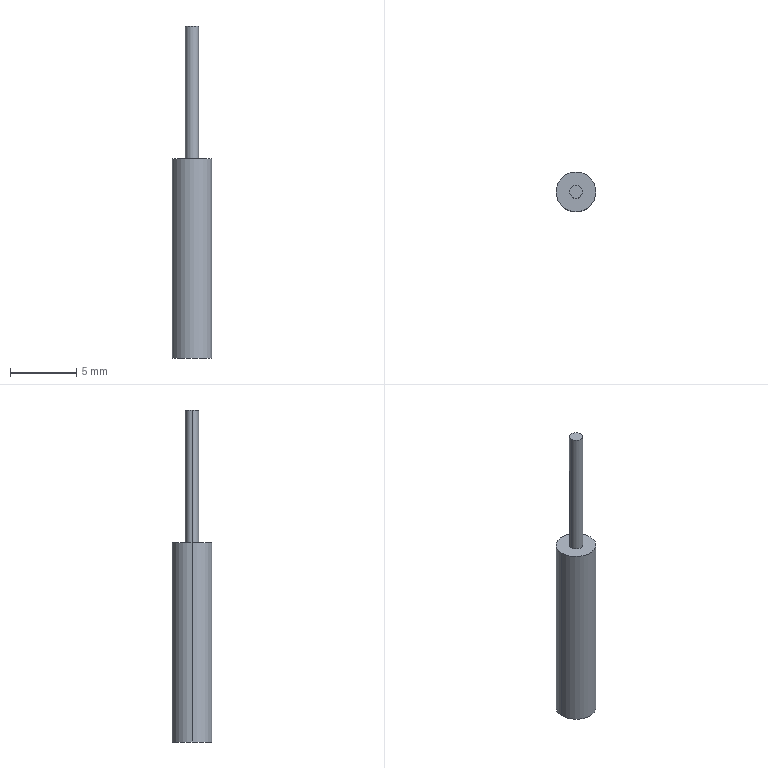Part | STEP file | Fiber sensor 1 | 1 solid | 7 faces | box 3 x 3 x 25 mm | volume 113.883 mm3 | cylinder 4 | plane 3 | commonest cylinder face diameters 1 x2 3 x2
STEP:
#1=CARTESIAN_POINT('',(0.,0.,0.));
#2=DIRECTION('',(0.,0.,1.));
#3=DIRECTION('',(1.,0.,0.));
#4=AXIS2_PLACEMENT_3D('',#1,#2,#3);
#5=CARTESIAN_POINT('',(-1.5,0.,-15.));
#6=VERTEX_POINT('',#5);
#7=CARTESIAN_POINT('',(1.5,0.,-15.));
#8=VERTEX_POINT('',#7);
#9=CARTESIAN_POINT('',(0.,0.,-15.));
#10=DIRECTION('',(0.,0.,-1.));
#11=DIRECTION('',(-1.,0.,0.));
#12=AXIS2_PLACEMENT_3D('',#9,#10,#11);
#13=CIRCLE('',#12,1.5);
#14=CARTESIAN_POINT('',(0.,0.,-15.));
#15=DIRECTION('',(0.,0.,1.));
#16=DIRECTION('',(1.,0.,0.));
#17=AXIS2_PLACEMENT_3D('',#14,#15,#16);
#18=CYLINDRICAL_SURFACE('',#17,1.5);
#19=CARTESIAN_POINT('',(3.142,0.));
#20=DIRECTION('',(-1.,0.));
#21=VECTOR('',#20,1.);
#22=LINE('',#19,#21);
#23=(GEOMETRIC_REPRESENTATION_CONTEXT(2)PARAMETRIC_REPRESENTATION_CONTEXT()REPRESENTATION_CONTEXT('',''));
#24=DEFINITIONAL_REPRESENTATION('',(#22),#23);
#25=PCURVE('',#18,#24);
#26=CARTESIAN_POINT('',(0.,0.,-15.));
#27=DIRECTION('',(0.,0.,-1.));
#28=DIRECTION('',(-1.,0.,0.));
#29=AXIS2_PLACEMENT_3D('',#26,#27,#28);
#30=PLANE('',#29);
#31=CARTESIAN_POINT('',(0.,0.));
#32=DIRECTION('',(1.,0.));
#33=AXIS2_PLACEMENT_2D('',#31,#32);
#34=CIRCLE('',#33,1.5);
#35=(GEOMETRIC_REPRESENTATION_CONTEXT(2)PARAMETRIC_REPRESENTATION_CONTEXT()REPRESENTATION_CONTEXT('',''));
#36=DEFINITIONAL_REPRESENTATION('',(#34),#35);
#37=PCURVE('',#30,#36);
#38=SURFACE_CURVE('',#13,(#25,#37),.PCURVE_S1.);
#39=EDGE_CURVE('',#6,#8,#38,.T.);
#40=ORIENTED_EDGE('',*,*,#39,.F.);
#41=CARTESIAN_POINT('',(-1.5,0.,0.));
#42=VERTEX_POINT('',#41);
#43=CARTESIAN_POINT('',(-1.5,0.,-15.));
#44=DIRECTION('',(0.,0.,1.));
#45=VECTOR('',#44,1.);
#46=LINE('',#43,#45);
#47=CARTESIAN_POINT('',(3.142,0.));
#48=DIRECTION('',(0.,1.));
#49=VECTOR('',#48,1.);
#50=LINE('',#47,#49);
#51=(GEOMETRIC_REPRESENTATION_CONTEXT(2)PARAMETRIC_REPRESENTATION_CONTEXT()REPRESENTATION_CONTEXT('',''));
#52=DEFINITIONAL_REPRESENTATION('',(#50),#51);
#53=PCURVE('',#18,#52);
#54=CARTESIAN_POINT('',(0.,0.,-15.));
#55=DIRECTION('',(0.,0.,1.));
#56=DIRECTION('',(1.,0.,0.));
#57=AXIS2_PLACEMENT_3D('',#54,#55,#56);
#58=CYLINDRICAL_SURFACE('',#57,1.5);
#59=CARTESIAN_POINT('',(3.142,0.));
#60=DIRECTION('',(0.,1.));
#61=VECTOR('',#60,1.);
#62=LINE('',#59,#61);
#63=(GEOMETRIC_REPRESENTATION_CONTEXT(2)PARAMETRIC_REPRESENTATION_CONTEXT()REPRESENTATION_CONTEXT('',''));
#64=DEFINITIONAL_REPRESENTATION('',(#62),#63);
#65=PCURVE('',#58,#64);
#66=SURFACE_CURVE('',#46,(#53,#65),.PCURVE_S1.);
#67=EDGE_CURVE('',#6,#42,#66,.T.);
#68=ORIENTED_EDGE('',*,*,#67,.T.);
#69=CARTESIAN_POINT('',(1.5,0.,0.));
#70=VERTEX_POINT('',#69);
#71=CARTESIAN_POINT('',(0.,0.,0.));
#72=DIRECTION('',(0.,0.,-1.));
#73=DIRECTION('',(-1.,0.,0.));
#74=AXIS2_PLACEMENT_3D('',#71,#72,#73);
#75=CIRCLE('',#74,1.5);
#76=CARTESIAN_POINT('',(3.142,15.));
#77=DIRECTION('',(-1.,0.));
#78=VECTOR('',#77,1.);
#79=LINE('',#76,#78);
#80=(GEOMETRIC_REPRESENTATION_CONTEXT(2)PARAMETRIC_REPRESENTATION_CONTEXT()REPRESENTATION_CONTEXT('',''));
#81=DEFINITIONAL_REPRESENTATION('',(#79),#80);
#82=PCURVE('',#18,#81);
#83=CARTESIAN_POINT('',(0.,0.,0.));
#84=DIRECTION('',(0.,0.,-1.));
#85=DIRECTION('',(-1.,0.,0.));
#86=AXIS2_PLACEMENT_3D('',#83,#84,#85);
#87=PLANE('',#86);
#88=CARTESIAN_POINT('',(0.,0.));
#89=DIRECTION('',(1.,0.));
#90=AXIS2_PLACEMENT_2D('',#88,#89);
#91=CIRCLE('',#90,1.5);
#92=(GEOMETRIC_REPRESENTATION_CONTEXT(2)PARAMETRIC_REPRESENTATION_CONTEXT()REPRESENTATION_CONTEXT('',''));
#93=DEFINITIONAL_REPRESENTATION('',(#91),#92);
#94=PCURVE('',#87,#93);
#95=SURFACE_CURVE('',#75,(#82,#94),.PCURVE_S1.);
#96=EDGE_CURVE('',#42,#70,#95,.T.);
#97=ORIENTED_EDGE('',*,*,#96,.T.);
#98=CARTESIAN_POINT('',(1.5,0.,-15.));
#99=DIRECTION('',(0.,0.,1.));
#100=VECTOR('',#99,1.);
#101=LINE('',#98,#100);
#102=CARTESIAN_POINT('',(0.,0.));
#103=DIRECTION('',(0.,1.));
#104=VECTOR('',#103,1.);
#105=LINE('',#102,#104);
#106=(GEOMETRIC_REPRESENTATION_CONTEXT(2)PARAMETRIC_REPRESENTATION_CONTEXT()REPRESENTATION_CONTEXT('',''));
#107=DEFINITIONAL_REPRESENTATION('',(#105),#106);
#108=PCURVE('',#18,#107);
#109=CARTESIAN_POINT('',(6.283,0.));
#110=DIRECTION('',(0.,1.));
#111=VECTOR('',#110,1.);
#112=LINE('',#109,#111);
#113=(GEOMETRIC_REPRESENTATION_CONTEXT(2)PARAMETRIC_REPRESENTATION_CONTEXT()REPRESENTATION_CONTEXT('',''));
#114=DEFINITIONAL_REPRESENTATION('',(#112),#113);
#115=PCURVE('',#58,#114);
#116=SURFACE_CURVE('',#101,(#108,#115),.PCURVE_S1.);
#117=EDGE_CURVE('',#8,#70,#116,.T.);
#118=ORIENTED_EDGE('',*,*,#117,.F.);
#119=EDGE_LOOP('',(#40,#68,#97,#118));
#120=FACE_BOUND('',#119,.T.);
#121=ADVANCED_FACE('',(#120),#18,.T.);
#122=CARTESIAN_POINT('',(0.5,0.,10.));
#123=VERTEX_POINT('',#122);
#124=CARTESIAN_POINT('',(-0.5,0.,10.));
#125=VERTEX_POINT('',#124);
#126=CARTESIAN_POINT('',(0.,0.,10.));
#127=DIRECTION('',(0.,0.,1.));
#128=DIRECTION('',(1.,0.,0.));
#129=AXIS2_PLACEMENT_3D('',#126,#127,#128);
#130=CIRCLE('',#129,0.5);
#131=CARTESIAN_POINT('',(0.,0.,10.));
#132=DIRECTION('',(0.,0.,-1.));
#133=DIRECTION('',(-1.,0.,0.));
#134=AXIS2_PLACEMENT_3D('',#131,#132,#133);
#135=CYLINDRICAL_SURFACE('',#134,0.5);
#136=CARTESIAN_POINT('',(3.142,0.));
#137=DIRECTION('',(-1.,0.));
#138=VECTOR('',#137,1.);
#139=LINE('',#136,#138);
#140=(GEOMETRIC_REPRESENTATION_CONTEXT(2)PARAMETRIC_REPRESENTATION_CONTEXT()REPRESENTATION_CONTEXT('',''));
#141=DEFINITIONAL_REPRESENTATION('',(#139),#140);
#142=PCURVE('',#135,#141);
#143=CARTESIAN_POINT('',(0.,0.,10.));
#144=DIRECTION('',(0.,0.,1.));
#145=DIRECTION('',(1.,0.,0.));
#146=AXIS2_PLACEMENT_3D('',#143,#144,#145);
#147=PLANE('',#146);
#148=CARTESIAN_POINT('',(0.,0.));
#149=DIRECTION('',(1.,0.));
#150=AXIS2_PLACEMENT_2D('',#148,#149);
#151=CIRCLE('',#150,0.5);
#152=(GEOMETRIC_REPRESENTATION_CONTEXT(2)PARAMETRIC_REPRESENTATION_CONTEXT()REPRESENTATION_CONTEXT('',''));
#153=DEFINITIONAL_REPRESENTATION('',(#151),#152);
#154=PCURVE('',#147,#153);
#155=SURFACE_CURVE('',#130,(#142,#154),.PCURVE_S1.);
#156=EDGE_CURVE('',#123,#125,#155,.T.);
#157=ORIENTED_EDGE('',*,*,#156,.F.);
#158=CARTESIAN_POINT('',(0.5,0.,0.));
#159=VERTEX_POINT('',#158);
#160=CARTESIAN_POINT('',(0.5,0.,10.));
#161=DIRECTION('',(0.,0.,-1.));
#162=VECTOR('',#161,1.);
#163=LINE('',#160,#162);
#164=CARTESIAN_POINT('',(3.142,0.));
#165=DIRECTION('',(0.,1.));
#166=VECTOR('',#165,1.);
#167=LINE('',#164,#166);
#168=(GEOMETRIC_REPRESENTATION_CONTEXT(2)PARAMETRIC_REPRESENTATION_CONTEXT()REPRESENTATION_CONTEXT('',''));
#169=DEFINITIONAL_REPRESENTATION('',(#167),#168);
#170=PCURVE('',#135,#169);
#171=CARTESIAN_POINT('',(0.,0.,10.));
#172=DIRECTION('',(0.,0.,-1.));
#173=DIRECTION('',(-1.,0.,0.));
#174=AXIS2_PLACEMENT_3D('',#171,#172,#173);
#175=CYLINDRICAL_SURFACE('',#174,0.5);
#176=CARTESIAN_POINT('',(3.142,0.));
#177=DIRECTION('',(0.,1.));
#178=VECTOR('',#177,1.);
#179=LINE('',#176,#178);
#180=(GEOMETRIC_REPRESENTATION_CONTEXT(2)PARAMETRIC_REPRESENTATION_CONTEXT()REPRESENTATION_CONTEXT('',''));
#181=DEFINITIONAL_REPRESENTATION('',(#179),#180);
#182=PCURVE('',#175,#181);
#183=SURFACE_CURVE('',#163,(#170,#182),.PCURVE_S1.);
#184=EDGE_CURVE('',#123,#159,#183,.T.);
#185=ORIENTED_EDGE('',*,*,#184,.T.);
#186=CARTESIAN_POINT('',(-0.5,0.,0.));
#187=VERTEX_POINT('',#186);
#188=CARTESIAN_POINT('',(0.,0.,0.));
#189=DIRECTION('',(0.,0.,-1.));
#190=DIRECTION('',(-1.,0.,0.));
#191=AXIS2_PLACEMENT_3D('',#188,#189,#190);
#192=CIRCLE('',#191,0.5);
#193=CARTESIAN_POINT('',(0.,10.));
#194=DIRECTION('',(1.,0.));
#195=VECTOR('',#194,1.);
#196=LINE('',#193,#195);
#197=(GEOMETRIC_REPRESENTATION_CONTEXT(2)PARAMETRIC_REPRESENTATION_CONTEXT()REPRESENTATION_CONTEXT('',''));
#198=DEFINITIONAL_REPRESENTATION('',(#196),#197);
#199=PCURVE('',#135,#198);
#200=CARTESIAN_POINT('',(0.,0.));
#201=DIRECTION('',(1.,0.));
#202=AXIS2_PLACEMENT_2D('',#200,#201);
#203=CIRCLE('',#202,0.5);
#204=(GEOMETRIC_REPRESENTATION_CONTEXT(2)PARAMETRIC_REPRESENTATION_CONTEXT()REPRESENTATION_CONTEXT('',''));
#205=DEFINITIONAL_REPRESENTATION('',(#203),#204);
#206=PCURVE('',#87,#205);
#207=SURFACE_CURVE('',#192,(#199,#206),.PCURVE_S1.);
#208=EDGE_CURVE('',#187,#159,#207,.T.);
#209=ORIENTED_EDGE('',*,*,#208,.F.);
#210=CARTESIAN_POINT('',(-0.5,0.,10.));
#211=DIRECTION('',(0.,0.,-1.));
#212=VECTOR('',#211,1.);
#213=LINE('',#210,#212);
#214=CARTESIAN_POINT('',(0.,0.));
#215=DIRECTION('',(0.,1.));
#216=VECTOR('',#215,1.);
#217=LINE('',#214,#216);
#218=(GEOMETRIC_REPRESENTATION_CONTEXT(2)PARAMETRIC_REPRESENTATION_CONTEXT()REPRESENTATION_CONTEXT('',''));
#219=DEFINITIONAL_REPRESENTATION('',(#217),#218);
#220=PCURVE('',#135,#219);
#221=CARTESIAN_POINT('',(6.283,0.));
#222=DIRECTION('',(0.,1.));
#223=VECTOR('',#222,1.);
#224=LINE('',#221,#223);
#225=(GEOMETRIC_REPRESENTATION_CONTEXT(2)PARAMETRIC_REPRESENTATION_CONTEXT()REPRESENTATION_CONTEXT('',''));
#226=DEFINITIONAL_REPRESENTATION('',(#224),#225);
#227=PCURVE('',#175,#226);
#228=SURFACE_CURVE('',#213,(#220,#227),.PCURVE_S1.);
#229=EDGE_CURVE('',#125,#187,#228,.T.);
#230=ORIENTED_EDGE('',*,*,#229,.F.);
#231=EDGE_LOOP('',(#157,#185,#209,#230));
#232=FACE_BOUND('',#231,.T.);
#233=ADVANCED_FACE('',(#232),#135,.T.);
#234=ORIENTED_EDGE('',*,*,#184,.F.);
#235=CARTESIAN_POINT('',(0.,0.,10.));
#236=DIRECTION('',(0.,0.,1.));
#237=DIRECTION('',(1.,0.,0.));
#238=AXIS2_PLACEMENT_3D('',#235,#236,#237);
#239=CIRCLE('',#238,0.5);
#240=CARTESIAN_POINT('',(9.425,0.));
#241=DIRECTION('',(-1.,0.));
#242=VECTOR('',#241,1.);
#243=LINE('',#240,#242);
#244=(GEOMETRIC_REPRESENTATION_CONTEXT(2)PARAMETRIC_REPRESENTATION_CONTEXT()REPRESENTATION_CONTEXT('',''));
#245=DEFINITIONAL_REPRESENTATION('',(#243),#244);
#246=PCURVE('',#175,#245);
#247=CARTESIAN_POINT('',(0.,0.));
#248=DIRECTION('',(1.,0.));
#249=AXIS2_PLACEMENT_2D('',#247,#248);
#250=CIRCLE('',#249,0.5);
#251=(GEOMETRIC_REPRESENTATION_CONTEXT(2)PARAMETRIC_REPRESENTATION_CONTEXT()REPRESENTATION_CONTEXT('',''));
#252=DEFINITIONAL_REPRESENTATION('',(#250),#251);
#253=PCURVE('',#147,#252);
#254=SURFACE_CURVE('',#239,(#246,#253),.PCURVE_S1.);
#255=EDGE_CURVE('',#125,#123,#254,.T.);
#256=ORIENTED_EDGE('',*,*,#255,.F.);
#257=ORIENTED_EDGE('',*,*,#229,.T.);
#258=CARTESIAN_POINT('',(0.,0.,0.));
#259=DIRECTION('',(0.,0.,-1.));
#260=DIRECTION('',(-1.,0.,0.));
#261=AXIS2_PLACEMENT_3D('',#258,#259,#260);
#262=CIRCLE('',#261,0.5);
#263=CARTESIAN_POINT('',(0.,10.));
#264=DIRECTION('',(1.,0.));
#265=VECTOR('',#264,1.);
#266=LINE('',#263,#265);
#267=(GEOMETRIC_REPRESENTATION_CONTEXT(2)PARAMETRIC_REPRESENTATION_CONTEXT()REPRESENTATION_CONTEXT('',''));
#268=DEFINITIONAL_REPRESENTATION('',(#266),#267);
#269=PCURVE('',#175,#268);
#270=CARTESIAN_POINT('',(0.,0.));
#271=DIRECTION('',(1.,0.));
#272=AXIS2_PLACEMENT_2D('',#270,#271);
#273=CIRCLE('',#272,0.5);
#274=(GEOMETRIC_REPRESENTATION_CONTEXT(2)PARAMETRIC_REPRESENTATION_CONTEXT()REPRESENTATION_CONTEXT('',''));
#275=DEFINITIONAL_REPRESENTATION('',(#273),#274);
#276=PCURVE('',#87,#275);
#277=SURFACE_CURVE('',#262,(#269,#276),.PCURVE_S1.);
#278=EDGE_CURVE('',#159,#187,#277,.T.);
#279=ORIENTED_EDGE('',*,*,#278,.F.);
#280=EDGE_LOOP('',(#234,#256,#257,#279));
#281=FACE_BOUND('',#280,.T.);
#282=ADVANCED_FACE('',(#281),#175,.T.);
#283=ORIENTED_EDGE('',*,*,#255,.T.);
#284=ORIENTED_EDGE('',*,*,#156,.T.);
#285=EDGE_LOOP('',(#283,#284));
#286=FACE_BOUND('',#285,.T.);
#287=ADVANCED_FACE('',(#286),#147,.T.);
#288=CARTESIAN_POINT('',(0.,0.,0.));
#289=DIRECTION('',(0.,0.,-1.));
#290=DIRECTION('',(-1.,0.,0.));
#291=AXIS2_PLACEMENT_3D('',#288,#289,#290);
#292=CIRCLE('',#291,1.5);
#293=CARTESIAN_POINT('',(0.,0.));
#294=DIRECTION('',(1.,0.));
#295=AXIS2_PLACEMENT_2D('',#293,#294);
#296=CIRCLE('',#295,1.5);
#297=(GEOMETRIC_REPRESENTATION_CONTEXT(2)PARAMETRIC_REPRESENTATION_CONTEXT()REPRESENTATION_CONTEXT('',''));
#298=DEFINITIONAL_REPRESENTATION('',(#296),#297);
#299=PCURVE('',#87,#298);
#300=CARTESIAN_POINT('',(9.425,15.));
#301=DIRECTION('',(-1.,0.));
#302=VECTOR('',#301,1.);
#303=LINE('',#300,#302);
#304=(GEOMETRIC_REPRESENTATION_CONTEXT(2)PARAMETRIC_REPRESENTATION_CONTEXT()REPRESENTATION_CONTEXT('',''));
#305=DEFINITIONAL_REPRESENTATION('',(#303),#304);
#306=PCURVE('',#58,#305);
#307=SURFACE_CURVE('',#292,(#299,#306),.PCURVE_S1.);
#308=EDGE_CURVE('',#70,#42,#307,.T.);
#309=ORIENTED_EDGE('',*,*,#308,.F.);
#310=ORIENTED_EDGE('',*,*,#96,.F.);
#311=EDGE_LOOP('',(#309,#310));
#312=FACE_BOUND('',#311,.T.);
#313=ORIENTED_EDGE('',*,*,#208,.T.);
#314=ORIENTED_EDGE('',*,*,#278,.T.);
#315=EDGE_LOOP('',(#313,#314));
#316=FACE_BOUND('',#315,.T.);
#317=ADVANCED_FACE('',(#312,#316),#87,.F.);
#318=ORIENTED_EDGE('',*,*,#67,.F.);
#319=CARTESIAN_POINT('',(0.,0.,-15.));
#320=DIRECTION('',(0.,0.,-1.));
#321=DIRECTION('',(-1.,0.,0.));
#322=AXIS2_PLACEMENT_3D('',#319,#320,#321);
#323=CIRCLE('',#322,1.5);
#324=CARTESIAN_POINT('',(9.425,0.));
#325=DIRECTION('',(-1.,0.));
#326=VECTOR('',#325,1.);
#327=LINE('',#324,#326);
#328=(GEOMETRIC_REPRESENTATION_CONTEXT(2)PARAMETRIC_REPRESENTATION_CONTEXT()REPRESENTATION_CONTEXT('',''));
#329=DEFINITIONAL_REPRESENTATION('',(#327),#328);
#330=PCURVE('',#58,#329);
#331=CARTESIAN_POINT('',(0.,0.));
#332=DIRECTION('',(1.,0.));
#333=AXIS2_PLACEMENT_2D('',#331,#332);
#334=CIRCLE('',#333,1.5);
#335=(GEOMETRIC_REPRESENTATION_CONTEXT(2)PARAMETRIC_REPRESENTATION_CONTEXT()REPRESENTATION_CONTEXT('',''));
#336=DEFINITIONAL_REPRESENTATION('',(#334),#335);
#337=PCURVE('',#30,#336);
#338=SURFACE_CURVE('',#323,(#330,#337),.PCURVE_S1.);
#339=EDGE_CURVE('',#8,#6,#338,.T.);
#340=ORIENTED_EDGE('',*,*,#339,.F.);
#341=ORIENTED_EDGE('',*,*,#117,.T.);
#342=ORIENTED_EDGE('',*,*,#308,.T.);
#343=EDGE_LOOP('',(#318,#340,#341,#342));
#344=FACE_BOUND('',#343,.T.);
#345=ADVANCED_FACE('',(#344),#58,.T.);
#346=ORIENTED_EDGE('',*,*,#339,.T.);
#347=ORIENTED_EDGE('',*,*,#39,.T.);
#348=EDGE_LOOP('',(#346,#347));
#349=FACE_BOUND('',#348,.T.);
#350=ADVANCED_FACE('',(#349),#30,.T.);
#351=CLOSED_SHELL('',(#121,#233,#282,#287,#317,#345,#350));
#352=MANIFOLD_SOLID_BREP('',#351);
#353=(LENGTH_UNIT()NAMED_UNIT(*)SI_UNIT(.MILLI.,.METRE.));
#354=UNCERTAINTY_MEASURE_WITH_UNIT(LENGTH_MEASURE(0.0000001),#353,'','');
#355=(NAMED_UNIT(*)PLANE_ANGLE_UNIT()SI_UNIT($,.RADIAN.));
#356=(NAMED_UNIT(*)SI_UNIT($,.STERADIAN.)SOLID_ANGLE_UNIT());
#357=(GEOMETRIC_REPRESENTATION_CONTEXT(3)GLOBAL_UNCERTAINTY_ASSIGNED_CONTEXT((#354))GLOBAL_UNIT_ASSIGNED_CONTEXT((#353,#355,#356))REPRESENTATION_CONTEXT('',''));
#358=ADVANCED_BREP_SHAPE_REPRESENTATION('',(#4,#352),#357);